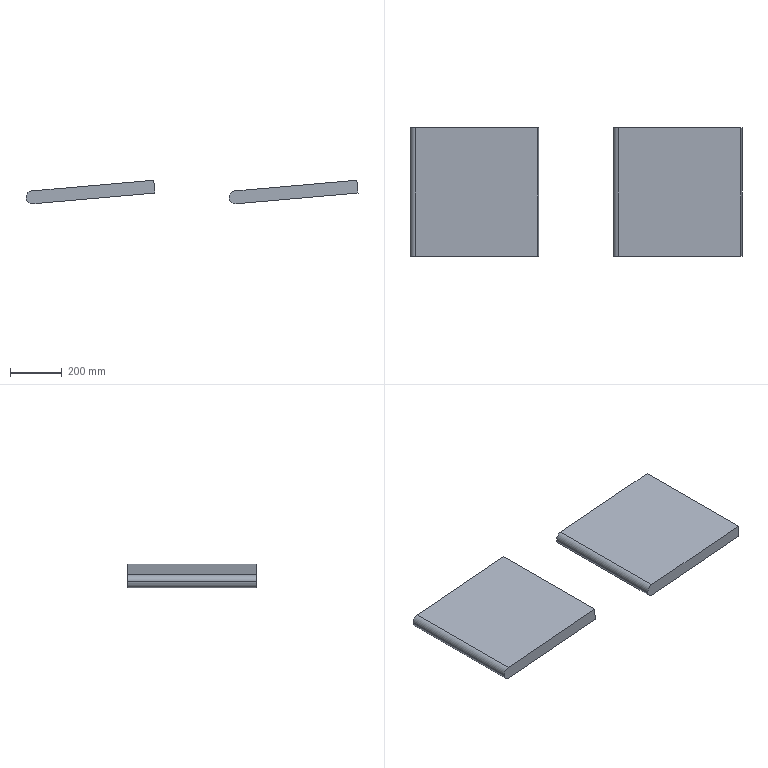Part | CATIA | 2 solids | 14 faces | box 1288 x 500 x 91.304 mm | volume 24731748 mm3 | plane 10 | cylinder 4 | commonest cylinder face diameters 50 x4
STEP:
#1=CARTESIAN_POINT('',(1350.,250.,60.));
#2=VERTEX_POINT('',#1);
#3=CARTESIAN_POINT('',(1823.192,250.,101.399));
#4=VERTEX_POINT('',#3);
#5=CARTESIAN_POINT('',(1586.596,250.,80.699));
#6=DIRECTION('',(0.9962,0.,0.08716));
#7=VECTOR('',#6,1.);
#8=LINE('',#5,#7);
#9=EDGE_CURVE('',#2,#4,#8,.T.);
#10=ORIENTED_EDGE('',*,*,#9,.F.);
#11=CARTESIAN_POINT('',(1350.,-250.,60.));
#12=VERTEX_POINT('',#11);
#13=CARTESIAN_POINT('',(1350.,0.,60.));
#14=DIRECTION('',(0.,-1.,0.));
#15=VECTOR('',#14,1.);
#16=LINE('',#13,#15);
#17=EDGE_CURVE('',#2,#12,#16,.T.);
#18=ORIENTED_EDGE('',*,*,#17,.T.);
#19=CARTESIAN_POINT('',(1823.192,-250.,101.399));
#20=VERTEX_POINT('',#19);
#21=CARTESIAN_POINT('',(1586.596,-250.,80.699));
#22=DIRECTION('',(-0.9962,0.,-0.08716));
#23=VECTOR('',#22,1.);
#24=LINE('',#21,#23);
#25=EDGE_CURVE('',#20,#12,#24,.T.);
#26=ORIENTED_EDGE('',*,*,#25,.F.);
#27=CARTESIAN_POINT('',(1823.192,0.,101.399));
#28=DIRECTION('',(0.,-1.,0.));
#29=VECTOR('',#28,1.);
#30=LINE('',#27,#29);
#31=EDGE_CURVE('',#4,#20,#30,.T.);
#32=ORIENTED_EDGE('',*,*,#31,.F.);
#33=EDGE_LOOP('',(#10,#18,#26,#32));
#34=FACE_OUTER_BOUND('',#33,.T.);
#35=CARTESIAN_POINT('',(1350.,0.,60.));
#36=DIRECTION('',(-0.08716,0.,0.9962));
#37=DIRECTION('',(0.9962,0.,0.08716));
#38=AXIS2_PLACEMENT_3D('',#35,#36,#37);
#39=PLANE('',#38);
#40=ADVANCED_FACE('',(#34),#39,.T.);
#41=CARTESIAN_POINT('',(1827.55,250.,51.589));
#42=VERTEX_POINT('',#41);
#43=CARTESIAN_POINT('',(1354.358,250.,10.19));
#44=VERTEX_POINT('',#43);
#45=CARTESIAN_POINT('',(1590.954,250.,30.89));
#46=DIRECTION('',(-0.9962,0.,-0.08716));
#47=VECTOR('',#46,1.);
#48=LINE('',#45,#47);
#49=EDGE_CURVE('',#42,#44,#48,.T.);
#50=ORIENTED_EDGE('',*,*,#49,.T.);
#51=CARTESIAN_POINT('',(1327.274,250.,32.916));
#52=VERTEX_POINT('',#51);
#53=CARTESIAN_POINT('',(1352.179,250.,35.095));
#54=DIRECTION('',(0.,1.,0.));
#55=AXIS2_PLACEMENT_3D('',#53,#54,$);
#56=CIRCLE('',#55,25.);
#57=EDGE_CURVE('',#44,#52,#56,.T.);
#58=ORIENTED_EDGE('',*,*,#57,.T.);
#59=CARTESIAN_POINT('',(1352.179,250.,35.095));
#60=DIRECTION('',(0.,1.,0.));
#61=AXIS2_PLACEMENT_3D('',#59,#60,$);
#62=CIRCLE('',#61,25.);
#63=EDGE_CURVE('',#52,#2,#62,.T.);
#64=ORIENTED_EDGE('',*,*,#63,.T.);
#65=ORIENTED_EDGE('',*,*,#9,.T.);
#66=CARTESIAN_POINT('',(1825.371,250.,76.494));
#67=DIRECTION('',(-0.08716,0.,0.9962));
#68=VECTOR('',#67,1.);
#69=LINE('',#66,#68);
#70=EDGE_CURVE('',#42,#4,#69,.T.);
#71=ORIENTED_EDGE('',*,*,#70,.F.);
#72=EDGE_LOOP('',(#50,#58,#64,#65,#71));
#73=FACE_OUTER_BOUND('',#72,.T.);
#74=CARTESIAN_POINT('',(1354.358,250.,10.19));
#75=DIRECTION('',(0.,1.,0.));
#76=DIRECTION('',(-0.08716,0.,0.9962));
#77=AXIS2_PLACEMENT_3D('',#74,#75,#76);
#78=PLANE('',#77);
#79=ADVANCED_FACE('',(#73),#78,.T.);
#80=ORIENTED_EDGE('',*,*,#17,.F.);
#81=ORIENTED_EDGE('',*,*,#63,.F.);
#82=CARTESIAN_POINT('',(1327.274,-250.,32.916));
#83=VERTEX_POINT('',#82);
#84=CARTESIAN_POINT('',(1327.274,0.,32.916));
#85=DIRECTION('',(0.,1.,0.));
#86=VECTOR('',#85,1.);
#87=LINE('',#84,#86);
#88=EDGE_CURVE('',#83,#52,#87,.T.);
#89=ORIENTED_EDGE('',*,*,#88,.F.);
#90=CARTESIAN_POINT('',(1352.179,-250.,35.095));
#91=DIRECTION('',(0.,1.,0.));
#92=AXIS2_PLACEMENT_3D('',#90,#91,$);
#93=CIRCLE('',#92,25.);
#94=EDGE_CURVE('',#12,#83,#93,.F.);
#95=ORIENTED_EDGE('',*,*,#94,.F.);
#96=EDGE_LOOP('',(#80,#81,#89,#95));
#97=FACE_OUTER_BOUND('',#96,.T.);
#98=CARTESIAN_POINT('',(1352.179,0.,35.095));
#99=DIRECTION('',(0.,1.,0.));
#100=DIRECTION('',(0.08716,0.,-0.9962));
#101=AXIS2_PLACEMENT_3D('',#98,#99,#100);
#102=CYLINDRICAL_SURFACE('',#101,25.);
#103=ADVANCED_FACE('',(#97),#102,.T.);
#104=ORIENTED_EDGE('',*,*,#94,.T.);
#105=CARTESIAN_POINT('',(1354.358,-250.,10.19));
#106=VERTEX_POINT('',#105);
#107=CARTESIAN_POINT('',(1352.179,-250.,35.095));
#108=DIRECTION('',(0.,-1.,0.));
#109=AXIS2_PLACEMENT_3D('',#107,#108,$);
#110=CIRCLE('',#109,25.);
#111=EDGE_CURVE('',#83,#106,#110,.T.);
#112=ORIENTED_EDGE('',*,*,#111,.T.);
#113=CARTESIAN_POINT('',(1827.55,-250.,51.589));
#114=VERTEX_POINT('',#113);
#115=CARTESIAN_POINT('',(1590.954,-250.,30.89));
#116=DIRECTION('',(0.9962,0.,0.08716));
#117=VECTOR('',#116,1.);
#118=LINE('',#115,#117);
#119=EDGE_CURVE('',#106,#114,#118,.T.);
#120=ORIENTED_EDGE('',*,*,#119,.T.);
#121=CARTESIAN_POINT('',(1825.371,-250.,76.494));
#122=DIRECTION('',(-0.08716,0.,0.9962));
#123=VECTOR('',#122,1.);
#124=LINE('',#121,#123);
#125=EDGE_CURVE('',#114,#20,#124,.T.);
#126=ORIENTED_EDGE('',*,*,#125,.T.);
#127=ORIENTED_EDGE('',*,*,#25,.T.);
#128=EDGE_LOOP('',(#104,#112,#120,#126,#127));
#129=FACE_OUTER_BOUND('',#128,.T.);
#130=CARTESIAN_POINT('',(1354.358,-250.,10.19));
#131=DIRECTION('',(0.,-1.,0.));
#132=DIRECTION('',(0.08716,0.,-0.9962));
#133=AXIS2_PLACEMENT_3D('',#130,#131,#132);
#134=PLANE('',#133);
#135=ADVANCED_FACE('',(#129),#134,.T.);
#136=CARTESIAN_POINT('',(1827.55,0.,51.589));
#137=DIRECTION('',(0.,1.,0.));
#138=VECTOR('',#137,1.);
#139=LINE('',#136,#138);
#140=EDGE_CURVE('',#114,#42,#139,.T.);
#141=ORIENTED_EDGE('',*,*,#140,.T.);
#142=ORIENTED_EDGE('',*,*,#70,.T.);
#143=ORIENTED_EDGE('',*,*,#31,.T.);
#144=ORIENTED_EDGE('',*,*,#125,.F.);
#145=EDGE_LOOP('',(#141,#142,#143,#144));
#146=FACE_OUTER_BOUND('',#145,.T.);
#147=CARTESIAN_POINT('',(1827.55,0.,51.589));
#148=DIRECTION('',(0.9962,0.,0.08716));
#149=DIRECTION('',(0.08716,0.,-0.9962));
#150=AXIS2_PLACEMENT_3D('',#147,#148,#149);
#151=PLANE('',#150);
#152=ADVANCED_FACE('',(#146),#151,.T.);
#153=ORIENTED_EDGE('',*,*,#119,.F.);
#154=CARTESIAN_POINT('',(1354.358,0.,10.19));
#155=DIRECTION('',(0.,1.,0.));
#156=VECTOR('',#155,1.);
#157=LINE('',#154,#156);
#158=EDGE_CURVE('',#106,#44,#157,.T.);
#159=ORIENTED_EDGE('',*,*,#158,.T.);
#160=ORIENTED_EDGE('',*,*,#49,.F.);
#161=ORIENTED_EDGE('',*,*,#140,.F.);
#162=EDGE_LOOP('',(#153,#159,#160,#161));
#163=FACE_OUTER_BOUND('',#162,.T.);
#164=CARTESIAN_POINT('',(1354.358,0.,10.19));
#165=DIRECTION('',(0.08716,0.,-0.9962));
#166=DIRECTION('',(-0.9962,0.,-0.08716));
#167=AXIS2_PLACEMENT_3D('',#164,#165,#166);
#168=PLANE('',#167);
#169=ADVANCED_FACE('',(#163),#168,.T.);
#170=ORIENTED_EDGE('',*,*,#57,.F.);
#171=ORIENTED_EDGE('',*,*,#158,.F.);
#172=ORIENTED_EDGE('',*,*,#111,.F.);
#173=ORIENTED_EDGE('',*,*,#88,.T.);
#174=EDGE_LOOP('',(#170,#171,#172,#173));
#175=FACE_OUTER_BOUND('',#174,.T.);
#176=CARTESIAN_POINT('',(1352.179,0.,35.095));
#177=DIRECTION('',(0.,-1.,0.));
#178=DIRECTION('',(-0.08716,0.,0.9962));
#179=AXIS2_PLACEMENT_3D('',#176,#177,#178);
#180=CYLINDRICAL_SURFACE('',#179,25.);
#181=ADVANCED_FACE('',(#175),#180,.T.);
#182=CLOSED_SHELL('',(#40,#79,#103,#135,#152,#169,#181));
#183=MANIFOLD_SOLID_BREP('',#182);
#184=CARTESIAN_POINT('',(562.,250.,60.));
#185=VERTEX_POINT('',#184);
#186=CARTESIAN_POINT('',(1035.192,250.,101.399));
#187=VERTEX_POINT('',#186);
#188=CARTESIAN_POINT('',(798.596,250.,80.699));
#189=DIRECTION('',(0.9962,0.,0.08716));
#190=VECTOR('',#189,1.);
#191=LINE('',#188,#190);
#192=EDGE_CURVE('',#185,#187,#191,.T.);
#193=ORIENTED_EDGE('',*,*,#192,.F.);
#194=CARTESIAN_POINT('',(562.,-250.,60.));
#195=VERTEX_POINT('',#194);
#196=CARTESIAN_POINT('',(562.,0.,60.));
#197=DIRECTION('',(0.,-1.,0.));
#198=VECTOR('',#197,1.);
#199=LINE('',#196,#198);
#200=EDGE_CURVE('',#185,#195,#199,.T.);
#201=ORIENTED_EDGE('',*,*,#200,.T.);
#202=CARTESIAN_POINT('',(1035.192,-250.,101.399));
#203=VERTEX_POINT('',#202);
#204=CARTESIAN_POINT('',(798.596,-250.,80.699));
#205=DIRECTION('',(-0.9962,0.,-0.08716));
#206=VECTOR('',#205,1.);
#207=LINE('',#204,#206);
#208=EDGE_CURVE('',#203,#195,#207,.T.);
#209=ORIENTED_EDGE('',*,*,#208,.F.);
#210=CARTESIAN_POINT('',(1035.192,0.,101.399));
#211=DIRECTION('',(0.,-1.,0.));
#212=VECTOR('',#211,1.);
#213=LINE('',#210,#212);
#214=EDGE_CURVE('',#187,#203,#213,.T.);
#215=ORIENTED_EDGE('',*,*,#214,.F.);
#216=EDGE_LOOP('',(#193,#201,#209,#215));
#217=FACE_OUTER_BOUND('',#216,.T.);
#218=CARTESIAN_POINT('',(562.,0.,60.));
#219=DIRECTION('',(-0.08716,0.,0.9962));
#220=DIRECTION('',(0.9962,0.,0.08716));
#221=AXIS2_PLACEMENT_3D('',#218,#219,#220);
#222=PLANE('',#221);
#223=ADVANCED_FACE('',(#217),#222,.T.);
#224=CARTESIAN_POINT('',(1039.55,250.,51.589));
#225=VERTEX_POINT('',#224);
#226=CARTESIAN_POINT('',(566.358,250.,10.19));
#227=VERTEX_POINT('',#226);
#228=CARTESIAN_POINT('',(802.954,250.,30.89));
#229=DIRECTION('',(-0.9962,0.,-0.08716));
#230=VECTOR('',#229,1.);
#231=LINE('',#228,#230);
#232=EDGE_CURVE('',#225,#227,#231,.T.);
#233=ORIENTED_EDGE('',*,*,#232,.T.);
#234=CARTESIAN_POINT('',(539.274,250.,32.916));
#235=VERTEX_POINT('',#234);
#236=CARTESIAN_POINT('',(564.179,250.,35.095));
#237=DIRECTION('',(0.,1.,0.));
#238=AXIS2_PLACEMENT_3D('',#236,#237,$);
#239=CIRCLE('',#238,25.);
#240=EDGE_CURVE('',#227,#235,#239,.T.);
#241=ORIENTED_EDGE('',*,*,#240,.T.);
#242=CARTESIAN_POINT('',(564.179,250.,35.095));
#243=DIRECTION('',(0.,1.,0.));
#244=AXIS2_PLACEMENT_3D('',#242,#243,$);
#245=CIRCLE('',#244,25.);
#246=EDGE_CURVE('',#235,#185,#245,.T.);
#247=ORIENTED_EDGE('',*,*,#246,.T.);
#248=ORIENTED_EDGE('',*,*,#192,.T.);
#249=CARTESIAN_POINT('',(1037.371,250.,76.494));
#250=DIRECTION('',(-0.08716,0.,0.9962));
#251=VECTOR('',#250,1.);
#252=LINE('',#249,#251);
#253=EDGE_CURVE('',#225,#187,#252,.T.);
#254=ORIENTED_EDGE('',*,*,#253,.F.);
#255=EDGE_LOOP('',(#233,#241,#247,#248,#254));
#256=FACE_OUTER_BOUND('',#255,.T.);
#257=CARTESIAN_POINT('',(566.358,250.,10.19));
#258=DIRECTION('',(0.,1.,0.));
#259=DIRECTION('',(-0.08716,0.,0.9962));
#260=AXIS2_PLACEMENT_3D('',#257,#258,#259);
#261=PLANE('',#260);
#262=ADVANCED_FACE('',(#256),#261,.T.);
#263=ORIENTED_EDGE('',*,*,#200,.F.);
#264=ORIENTED_EDGE('',*,*,#246,.F.);
#265=CARTESIAN_POINT('',(539.274,-250.,32.916));
#266=VERTEX_POINT('',#265);
#267=CARTESIAN_POINT('',(539.274,0.,32.916));
#268=DIRECTION('',(0.,1.,0.));
#269=VECTOR('',#268,1.);
#270=LINE('',#267,#269);
#271=EDGE_CURVE('',#266,#235,#270,.T.);
#272=ORIENTED_EDGE('',*,*,#271,.F.);
#273=CARTESIAN_POINT('',(564.179,-250.,35.095));
#274=DIRECTION('',(0.,1.,0.));
#275=AXIS2_PLACEMENT_3D('',#273,#274,$);
#276=CIRCLE('',#275,25.);
#277=EDGE_CURVE('',#195,#266,#276,.F.);
#278=ORIENTED_EDGE('',*,*,#277,.F.);
#279=EDGE_LOOP('',(#263,#264,#272,#278));
#280=FACE_OUTER_BOUND('',#279,.T.);
#281=CARTESIAN_POINT('',(564.179,0.,35.095));
#282=DIRECTION('',(0.,1.,0.));
#283=DIRECTION('',(0.08716,0.,-0.9962));
#284=AXIS2_PLACEMENT_3D('',#281,#282,#283);
#285=CYLINDRICAL_SURFACE('',#284,25.);
#286=ADVANCED_FACE('',(#280),#285,.T.);
#287=ORIENTED_EDGE('',*,*,#277,.T.);
#288=CARTESIAN_POINT('',(566.358,-250.,10.19));
#289=VERTEX_POINT('',#288);
#290=CARTESIAN_POINT('',(564.179,-250.,35.095));
#291=DIRECTION('',(0.,-1.,0.));
#292=AXIS2_PLACEMENT_3D('',#290,#291,$);
#293=CIRCLE('',#292,25.);
#294=EDGE_CURVE('',#266,#289,#293,.T.);
#295=ORIENTED_EDGE('',*,*,#294,.T.);
#296=CARTESIAN_POINT('',(1039.55,-250.,51.589));
#297=VERTEX_POINT('',#296);
#298=CARTESIAN_POINT('',(802.954,-250.,30.89));
#299=DIRECTION('',(0.9962,0.,0.08716));
#300=VECTOR('',#299,1.);
#301=LINE('',#298,#300);
#302=EDGE_CURVE('',#289,#297,#301,.T.);
#303=ORIENTED_EDGE('',*,*,#302,.T.);
#304=CARTESIAN_POINT('',(1037.371,-250.,76.494));
#305=DIRECTION('',(-0.08716,0.,0.9962));
#306=VECTOR('',#305,1.);
#307=LINE('',#304,#306);
#308=EDGE_CURVE('',#297,#203,#307,.T.);
#309=ORIENTED_EDGE('',*,*,#308,.T.);
#310=ORIENTED_EDGE('',*,*,#208,.T.);
#311=EDGE_LOOP('',(#287,#295,#303,#309,#310));
#312=FACE_OUTER_BOUND('',#311,.T.);
#313=CARTESIAN_POINT('',(566.358,-250.,10.19));
#314=DIRECTION('',(0.,-1.,0.));
#315=DIRECTION('',(0.08716,0.,-0.9962));
#316=AXIS2_PLACEMENT_3D('',#313,#314,#315);
#317=PLANE('',#316);
#318=ADVANCED_FACE('',(#312),#317,.T.);
#319=CARTESIAN_POINT('',(1039.55,0.,51.589));
#320=DIRECTION('',(0.,1.,0.));
#321=VECTOR('',#320,1.);
#322=LINE('',#319,#321);
#323=EDGE_CURVE('',#297,#225,#322,.T.);
#324=ORIENTED_EDGE('',*,*,#323,.T.);
#325=ORIENTED_EDGE('',*,*,#253,.T.);
#326=ORIENTED_EDGE('',*,*,#214,.T.);
#327=ORIENTED_EDGE('',*,*,#308,.F.);
#328=EDGE_LOOP('',(#324,#325,#326,#327));
#329=FACE_OUTER_BOUND('',#328,.T.);
#330=CARTESIAN_POINT('',(1039.55,0.,51.589));
#331=DIRECTION('',(0.9962,0.,0.08716));
#332=DIRECTION('',(0.08716,0.,-0.9962));
#333=AXIS2_PLACEMENT_3D('',#330,#331,#332);
#334=PLANE('',#333);
#335=ADVANCED_FACE('',(#329),#334,.T.);
#336=ORIENTED_EDGE('',*,*,#302,.F.);
#337=CARTESIAN_POINT('',(566.358,0.,10.19));
#338=DIRECTION('',(0.,1.,0.));
#339=VECTOR('',#338,1.);
#340=LINE('',#337,#339);
#341=EDGE_CURVE('',#289,#227,#340,.T.);
#342=ORIENTED_EDGE('',*,*,#341,.T.);
#343=ORIENTED_EDGE('',*,*,#232,.F.);
#344=ORIENTED_EDGE('',*,*,#323,.F.);
#345=EDGE_LOOP('',(#336,#342,#343,#344));
#346=FACE_OUTER_BOUND('',#345,.T.);
#347=CARTESIAN_POINT('',(566.358,0.,10.19));
#348=DIRECTION('',(0.08716,0.,-0.9962));
#349=DIRECTION('',(-0.9962,0.,-0.08716));
#350=AXIS2_PLACEMENT_3D('',#347,#348,#349);
#351=PLANE('',#350);
#352=ADVANCED_FACE('',(#346),#351,.T.);
#353=ORIENTED_EDGE('',*,*,#240,.F.);
#354=ORIENTED_EDGE('',*,*,#341,.F.);
#355=ORIENTED_EDGE('',*,*,#294,.F.);
#356=ORIENTED_EDGE('',*,*,#271,.T.);
#357=EDGE_LOOP('',(#353,#354,#355,#356));
#358=FACE_OUTER_BOUND('',#357,.T.);
#359=CARTESIAN_POINT('',(564.179,0.,35.095));
#360=DIRECTION('',(0.,-1.,0.));
#361=DIRECTION('',(-0.08716,0.,0.9962));
#362=AXIS2_PLACEMENT_3D('',#359,#360,#361);
#363=CYLINDRICAL_SURFACE('',#362,25.);
#364=ADVANCED_FACE('',(#358),#363,.T.);
#365=CLOSED_SHELL('',(#223,#262,#286,#318,#335,#352,#364));
#366=MANIFOLD_SOLID_BREP('',#365);
#367=(LENGTH_UNIT()NAMED_UNIT(*)SI_UNIT(.MILLI.,.METRE.));
#368=UNCERTAINTY_MEASURE_WITH_UNIT(LENGTH_MEASURE(0.005),#367,'','');
#369=(NAMED_UNIT(*)PLANE_ANGLE_UNIT()SI_UNIT($,.RADIAN.));
#370=(NAMED_UNIT(*)SI_UNIT($,.STERADIAN.)SOLID_ANGLE_UNIT());
#371=(GEOMETRIC_REPRESENTATION_CONTEXT(3)GLOBAL_UNCERTAINTY_ASSIGNED_CONTEXT((#368))GLOBAL_UNIT_ASSIGNED_CONTEXT((#367,#369,#370))REPRESENTATION_CONTEXT('',''));
#372=ADVANCED_BREP_SHAPE_REPRESENTATION('',(#183,#366),#371);